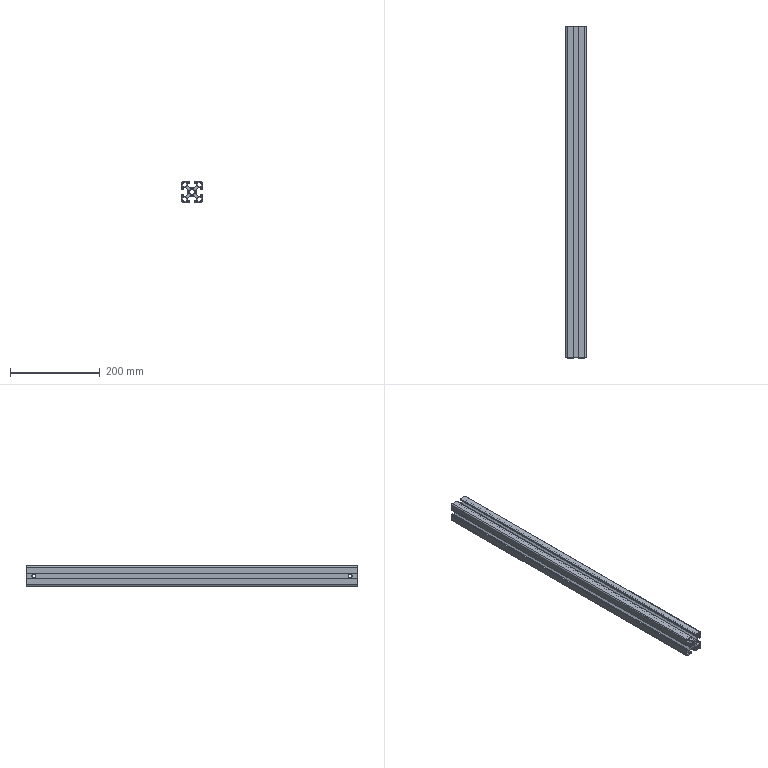Part | STEP file | 1 solid | 179 faces | box 45 x 738 x 45 mm | volume 510078 mm3 | plane 142 | cylinder 37 | commonest cylinder face diameters 10 x21 9 x8 3 x4 5 x4